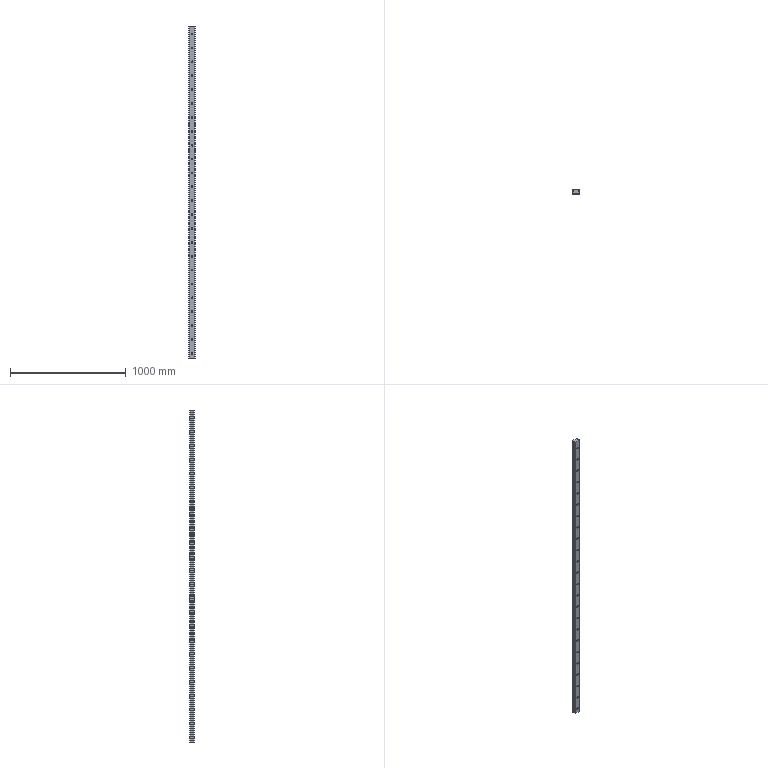Part | Creo | features CUT 48, CURVE 3, DATUM PLANE 3, PATTERN 2, CHAMFER 1, COORDINATE SYSTEM 1, PROTRUSION 1 | 1 solid | 134 faces | box 53 x 38 x 2870 mm | volume 5298046 mm3 | cylinder 98 | plane 36 | commonest cylinder face diameters 15 x48 23 x48 8.877 x2